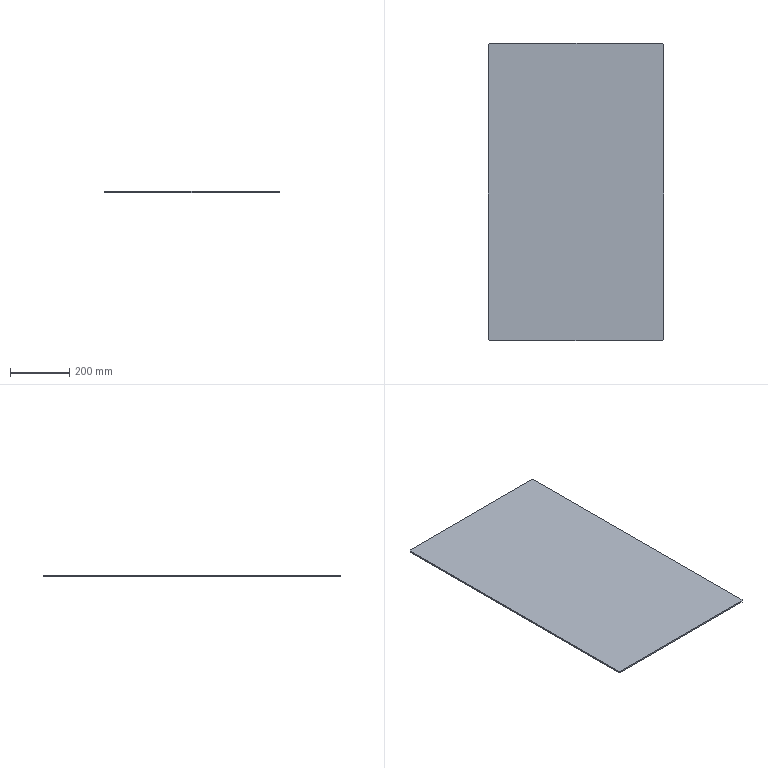Part | SolidWorks | features Chamfer 1, Extrusion 1 | 1 solid | 10 faces | box 590 x 1000 x 5 mm | volume 2949750 mm3 | plane 10
STEP:
#1=CARTESIAN_POINT('',(-295.,495.,0.));
#2=VERTEX_POINT('',#1);
#3=CARTESIAN_POINT('',(-295.,-495.,0.));
#4=VERTEX_POINT('',#3);
#5=CARTESIAN_POINT('',(-295.,500.,0.));
#6=DIRECTION('',(0.,-1.,0.));
#7=VECTOR('',#6,1000.);
#8=LINE('',#5,#7);
#9=EDGE_CURVE('',#2,#4,#8,.T.);
#10=ORIENTED_EDGE('',*,*,#9,.T.);
#11=CARTESIAN_POINT('',(-295.,-495.,5.));
#12=VERTEX_POINT('',#11);
#13=CARTESIAN_POINT('',(-295.,-495.,5.));
#14=DIRECTION('',(0.,0.,1.));
#15=VECTOR('',#14,1000.);
#16=LINE('',#13,#15);
#17=EDGE_CURVE('',#4,#12,#16,.T.);
#18=ORIENTED_EDGE('',*,*,#17,.T.);
#19=CARTESIAN_POINT('',(-295.,495.,5.));
#20=VERTEX_POINT('',#19);
#21=CARTESIAN_POINT('',(-295.,500.,5.));
#22=DIRECTION('',(0.,-1.,0.));
#23=VECTOR('',#22,1000.);
#24=LINE('',#21,#23);
#25=EDGE_CURVE('',#20,#12,#24,.T.);
#26=ORIENTED_EDGE('',*,*,#25,.F.);
#27=CARTESIAN_POINT('',(-295.,495.,5.));
#28=DIRECTION('',(0.,0.,-1.));
#29=VECTOR('',#28,1000.);
#30=LINE('',#27,#29);
#31=EDGE_CURVE('',#20,#2,#30,.T.);
#32=ORIENTED_EDGE('',*,*,#31,.T.);
#33=EDGE_LOOP('',(#10,#18,#26,#32));
#34=FACE_OUTER_BOUND('',#33,.T.);
#35=CARTESIAN_POINT('',(-295.,500.,5.));
#36=DIRECTION('',(1.,0.,0.));
#37=DIRECTION('',(0.,1.,0.));
#38=AXIS2_PLACEMENT_3D('',#35,#36,#37);
#39=PLANE('',#38);
#40=ADVANCED_FACE('',(#34),#39,.F.);
#41=CARTESIAN_POINT('',(-290.,-500.,5.));
#42=VERTEX_POINT('',#41);
#43=CARTESIAN_POINT('',(290.,-500.,5.));
#44=VERTEX_POINT('',#43);
#45=CARTESIAN_POINT('',(-295.,-500.,5.));
#46=DIRECTION('',(1.,0.,0.));
#47=VECTOR('',#46,1000.);
#48=LINE('',#45,#47);
#49=EDGE_CURVE('',#42,#44,#48,.T.);
#50=ORIENTED_EDGE('',*,*,#49,.F.);
#51=CARTESIAN_POINT('',(-290.,-500.,0.));
#52=VERTEX_POINT('',#51);
#53=CARTESIAN_POINT('',(-290.,-500.,5.));
#54=DIRECTION('',(0.,0.,-1.));
#55=VECTOR('',#54,1000.);
#56=LINE('',#53,#55);
#57=EDGE_CURVE('',#42,#52,#56,.T.);
#58=ORIENTED_EDGE('',*,*,#57,.T.);
#59=CARTESIAN_POINT('',(290.,-500.,0.));
#60=VERTEX_POINT('',#59);
#61=CARTESIAN_POINT('',(-295.,-500.,0.));
#62=DIRECTION('',(1.,0.,0.));
#63=VECTOR('',#62,1000.);
#64=LINE('',#61,#63);
#65=EDGE_CURVE('',#52,#60,#64,.T.);
#66=ORIENTED_EDGE('',*,*,#65,.T.);
#67=CARTESIAN_POINT('',(290.,-500.,5.));
#68=DIRECTION('',(0.,0.,1.));
#69=VECTOR('',#68,1000.);
#70=LINE('',#67,#69);
#71=EDGE_CURVE('',#60,#44,#70,.T.);
#72=ORIENTED_EDGE('',*,*,#71,.T.);
#73=EDGE_LOOP('',(#50,#58,#66,#72));
#74=FACE_OUTER_BOUND('',#73,.T.);
#75=CARTESIAN_POINT('',(-295.,-500.,5.));
#76=DIRECTION('',(0.,1.,0.));
#77=DIRECTION('',(0.,0.,1.));
#78=AXIS2_PLACEMENT_3D('',#75,#76,#77);
#79=PLANE('',#78);
#80=ADVANCED_FACE('',(#74),#79,.F.);
#81=CARTESIAN_POINT('',(295.,-495.,5.));
#82=VERTEX_POINT('',#81);
#83=CARTESIAN_POINT('',(295.,495.,5.));
#84=VERTEX_POINT('',#83);
#85=CARTESIAN_POINT('',(295.,500.,5.));
#86=DIRECTION('',(0.,1.,0.));
#87=VECTOR('',#86,1000.);
#88=LINE('',#85,#87);
#89=EDGE_CURVE('',#82,#84,#88,.T.);
#90=ORIENTED_EDGE('',*,*,#89,.F.);
#91=CARTESIAN_POINT('',(295.,-495.,0.));
#92=VERTEX_POINT('',#91);
#93=CARTESIAN_POINT('',(295.,-495.,5.));
#94=DIRECTION('',(0.,0.,-1.));
#95=VECTOR('',#94,1000.);
#96=LINE('',#93,#95);
#97=EDGE_CURVE('',#82,#92,#96,.T.);
#98=ORIENTED_EDGE('',*,*,#97,.T.);
#99=CARTESIAN_POINT('',(295.,495.,0.));
#100=VERTEX_POINT('',#99);
#101=CARTESIAN_POINT('',(295.,500.,0.));
#102=DIRECTION('',(0.,1.,0.));
#103=VECTOR('',#102,1000.);
#104=LINE('',#101,#103);
#105=EDGE_CURVE('',#92,#100,#104,.T.);
#106=ORIENTED_EDGE('',*,*,#105,.T.);
#107=CARTESIAN_POINT('',(295.,495.,5.));
#108=DIRECTION('',(0.,0.,1.));
#109=VECTOR('',#108,1000.);
#110=LINE('',#107,#109);
#111=EDGE_CURVE('',#100,#84,#110,.T.);
#112=ORIENTED_EDGE('',*,*,#111,.T.);
#113=EDGE_LOOP('',(#90,#98,#106,#112));
#114=FACE_OUTER_BOUND('',#113,.T.);
#115=CARTESIAN_POINT('',(295.,500.,5.));
#116=DIRECTION('',(-1.,0.,0.));
#117=DIRECTION('',(0.,-1.,0.));
#118=AXIS2_PLACEMENT_3D('',#115,#116,#117);
#119=PLANE('',#118);
#120=ADVANCED_FACE('',(#114),#119,.F.);
#121=CARTESIAN_POINT('',(290.,500.,5.));
#122=VERTEX_POINT('',#121);
#123=CARTESIAN_POINT('',(-290.,500.,5.));
#124=VERTEX_POINT('',#123);
#125=CARTESIAN_POINT('',(-295.,500.,5.));
#126=DIRECTION('',(-1.,0.,0.));
#127=VECTOR('',#126,1000.);
#128=LINE('',#125,#127);
#129=EDGE_CURVE('',#122,#124,#128,.T.);
#130=ORIENTED_EDGE('',*,*,#129,.F.);
#131=CARTESIAN_POINT('',(290.,500.,0.));
#132=VERTEX_POINT('',#131);
#133=CARTESIAN_POINT('',(290.,500.,5.));
#134=DIRECTION('',(0.,0.,-1.));
#135=VECTOR('',#134,1000.);
#136=LINE('',#133,#135);
#137=EDGE_CURVE('',#122,#132,#136,.T.);
#138=ORIENTED_EDGE('',*,*,#137,.T.);
#139=CARTESIAN_POINT('',(-290.,500.,0.));
#140=VERTEX_POINT('',#139);
#141=CARTESIAN_POINT('',(-295.,500.,0.));
#142=DIRECTION('',(-1.,0.,0.));
#143=VECTOR('',#142,1000.);
#144=LINE('',#141,#143);
#145=EDGE_CURVE('',#132,#140,#144,.T.);
#146=ORIENTED_EDGE('',*,*,#145,.T.);
#147=CARTESIAN_POINT('',(-290.,500.,5.));
#148=DIRECTION('',(0.,0.,1.));
#149=VECTOR('',#148,1000.);
#150=LINE('',#147,#149);
#151=EDGE_CURVE('',#140,#124,#150,.T.);
#152=ORIENTED_EDGE('',*,*,#151,.T.);
#153=EDGE_LOOP('',(#130,#138,#146,#152));
#154=FACE_OUTER_BOUND('',#153,.T.);
#155=CARTESIAN_POINT('',(-295.,500.,5.));
#156=DIRECTION('',(0.,-1.,0.));
#157=DIRECTION('',(0.,0.,-1.));
#158=AXIS2_PLACEMENT_3D('',#155,#156,#157);
#159=PLANE('',#158);
#160=ADVANCED_FACE('',(#154),#159,.F.);
#161=ORIENTED_EDGE('',*,*,#25,.T.);
#162=CARTESIAN_POINT('',(-292.5,-497.5,5.));
#163=DIRECTION('',(0.7071,-0.7071,0.));
#164=VECTOR('',#163,1000.);
#165=LINE('',#162,#164);
#166=EDGE_CURVE('',#12,#42,#165,.T.);
#167=ORIENTED_EDGE('',*,*,#166,.T.);
#168=ORIENTED_EDGE('',*,*,#49,.T.);
#169=CARTESIAN_POINT('',(-2.5,-792.5,5.));
#170=DIRECTION('',(0.7071,0.7071,0.));
#171=VECTOR('',#170,1000.);
#172=LINE('',#169,#171);
#173=EDGE_CURVE('',#44,#82,#172,.T.);
#174=ORIENTED_EDGE('',*,*,#173,.T.);
#175=ORIENTED_EDGE('',*,*,#89,.T.);
#176=CARTESIAN_POINT('',(497.5,292.5,5.));
#177=DIRECTION('',(-0.7071,0.7071,0.));
#178=VECTOR('',#177,1000.);
#179=LINE('',#176,#178);
#180=EDGE_CURVE('',#84,#122,#179,.T.);
#181=ORIENTED_EDGE('',*,*,#180,.T.);
#182=ORIENTED_EDGE('',*,*,#129,.T.);
#183=CARTESIAN_POINT('',(-792.5,-2.5,5.));
#184=DIRECTION('',(-0.7071,-0.7071,0.));
#185=VECTOR('',#184,1000.);
#186=LINE('',#183,#185);
#187=EDGE_CURVE('',#124,#20,#186,.T.);
#188=ORIENTED_EDGE('',*,*,#187,.T.);
#189=EDGE_LOOP('',(#161,#167,#168,#174,#175,#181,#182,#188));
#190=FACE_OUTER_BOUND('',#189,.T.);
#191=CARTESIAN_POINT('',(-295.,-500.,5.));
#192=DIRECTION('',(0.,0.,1.));
#193=DIRECTION('',(1.,0.,0.));
#194=AXIS2_PLACEMENT_3D('',#191,#192,#193);
#195=PLANE('',#194);
#196=ADVANCED_FACE('',(#190),#195,.T.);
#197=ORIENTED_EDGE('',*,*,#65,.F.);
#198=CARTESIAN_POINT('',(-290.,-500.,0.));
#199=DIRECTION('',(-0.7071,0.7071,0.));
#200=VECTOR('',#199,1000.);
#201=LINE('',#198,#200);
#202=EDGE_CURVE('',#52,#4,#201,.T.);
#203=ORIENTED_EDGE('',*,*,#202,.T.);
#204=ORIENTED_EDGE('',*,*,#9,.F.);
#205=CARTESIAN_POINT('',(-295.,495.,0.));
#206=DIRECTION('',(0.7071,0.7071,0.));
#207=VECTOR('',#206,1000.);
#208=LINE('',#205,#207);
#209=EDGE_CURVE('',#2,#140,#208,.T.);
#210=ORIENTED_EDGE('',*,*,#209,.T.);
#211=ORIENTED_EDGE('',*,*,#145,.F.);
#212=CARTESIAN_POINT('',(290.,500.,0.));
#213=DIRECTION('',(0.7071,-0.7071,0.));
#214=VECTOR('',#213,1000.);
#215=LINE('',#212,#214);
#216=EDGE_CURVE('',#132,#100,#215,.T.);
#217=ORIENTED_EDGE('',*,*,#216,.T.);
#218=ORIENTED_EDGE('',*,*,#105,.F.);
#219=CARTESIAN_POINT('',(295.,-495.,0.));
#220=DIRECTION('',(-0.7071,-0.7071,0.));
#221=VECTOR('',#220,1000.);
#222=LINE('',#219,#221);
#223=EDGE_CURVE('',#92,#60,#222,.T.);
#224=ORIENTED_EDGE('',*,*,#223,.T.);
#225=EDGE_LOOP('',(#197,#203,#204,#210,#211,#217,#218,#224));
#226=FACE_OUTER_BOUND('',#225,.T.);
#227=CARTESIAN_POINT('',(-295.,-500.,0.));
#228=DIRECTION('',(0.,0.,1.));
#229=DIRECTION('',(1.,0.,0.));
#230=AXIS2_PLACEMENT_3D('',#227,#228,#229);
#231=PLANE('',#230);
#232=ADVANCED_FACE('',(#226),#231,.F.);
#233=ORIENTED_EDGE('',*,*,#166,.F.);
#234=ORIENTED_EDGE('',*,*,#17,.F.);
#235=ORIENTED_EDGE('',*,*,#202,.F.);
#236=ORIENTED_EDGE('',*,*,#57,.F.);
#237=EDGE_LOOP('',(#233,#234,#235,#236));
#238=FACE_OUTER_BOUND('',#237,.T.);
#239=CARTESIAN_POINT('',(-290.,-500.,5.));
#240=DIRECTION('',(0.7071,0.7071,0.));
#241=DIRECTION('',(-0.7071,0.7071,0.));
#242=AXIS2_PLACEMENT_3D('',#239,#240,#241);
#243=PLANE('',#242);
#244=ADVANCED_FACE('',(#238),#243,.F.);
#245=ORIENTED_EDGE('',*,*,#173,.F.);
#246=ORIENTED_EDGE('',*,*,#71,.F.);
#247=ORIENTED_EDGE('',*,*,#223,.F.);
#248=ORIENTED_EDGE('',*,*,#97,.F.);
#249=EDGE_LOOP('',(#245,#246,#247,#248));
#250=FACE_OUTER_BOUND('',#249,.T.);
#251=CARTESIAN_POINT('',(295.,-495.,5.));
#252=DIRECTION('',(-0.7071,0.7071,0.));
#253=DIRECTION('',(-0.7071,-0.7071,0.));
#254=AXIS2_PLACEMENT_3D('',#251,#252,#253);
#255=PLANE('',#254);
#256=ADVANCED_FACE('',(#250),#255,.F.);
#257=ORIENTED_EDGE('',*,*,#180,.F.);
#258=ORIENTED_EDGE('',*,*,#111,.F.);
#259=ORIENTED_EDGE('',*,*,#216,.F.);
#260=ORIENTED_EDGE('',*,*,#137,.F.);
#261=EDGE_LOOP('',(#257,#258,#259,#260));
#262=FACE_OUTER_BOUND('',#261,.T.);
#263=CARTESIAN_POINT('',(290.,500.,5.));
#264=DIRECTION('',(-0.7071,-0.7071,0.));
#265=DIRECTION('',(0.7071,-0.7071,0.));
#266=AXIS2_PLACEMENT_3D('',#263,#264,#265);
#267=PLANE('',#266);
#268=ADVANCED_FACE('',(#262),#267,.F.);
#269=ORIENTED_EDGE('',*,*,#187,.F.);
#270=ORIENTED_EDGE('',*,*,#151,.F.);
#271=ORIENTED_EDGE('',*,*,#209,.F.);
#272=ORIENTED_EDGE('',*,*,#31,.F.);
#273=EDGE_LOOP('',(#269,#270,#271,#272));
#274=FACE_OUTER_BOUND('',#273,.T.);
#275=CARTESIAN_POINT('',(-295.,495.,5.));
#276=DIRECTION('',(0.7071,-0.7071,0.));
#277=DIRECTION('',(0.7071,0.7071,0.));
#278=AXIS2_PLACEMENT_3D('',#275,#276,#277);
#279=PLANE('',#278);
#280=ADVANCED_FACE('',(#274),#279,.F.);
#281=CLOSED_SHELL('',(#40,#80,#120,#160,#196,#232,#244,#256,#268,#280));
#282=MANIFOLD_SOLID_BREP('',#281);
#283=CARTESIAN_POINT('',(0.,0.,0.));
#284=DIRECTION('',(0.,0.,1.));
#285=DIRECTION('',(1.,0.,0.));
#286=AXIS2_PLACEMENT_3D('',#283,#284,#285);
#287=(LENGTH_UNIT()NAMED_UNIT(*)SI_UNIT(.MILLI.,.METRE.));
#288=UNCERTAINTY_MEASURE_WITH_UNIT(LENGTH_MEASURE(0.00001),#287,'','');
#289=(NAMED_UNIT(*)PLANE_ANGLE_UNIT()SI_UNIT($,.RADIAN.));
#290=(NAMED_UNIT(*)SI_UNIT($,.STERADIAN.)SOLID_ANGLE_UNIT());
#291=(GEOMETRIC_REPRESENTATION_CONTEXT(3)GLOBAL_UNCERTAINTY_ASSIGNED_CONTEXT((#288))GLOBAL_UNIT_ASSIGNED_CONTEXT((#287,#289,#290))REPRESENTATION_CONTEXT('',''));
#292=ADVANCED_BREP_SHAPE_REPRESENTATION('',(#282,#286),#291);